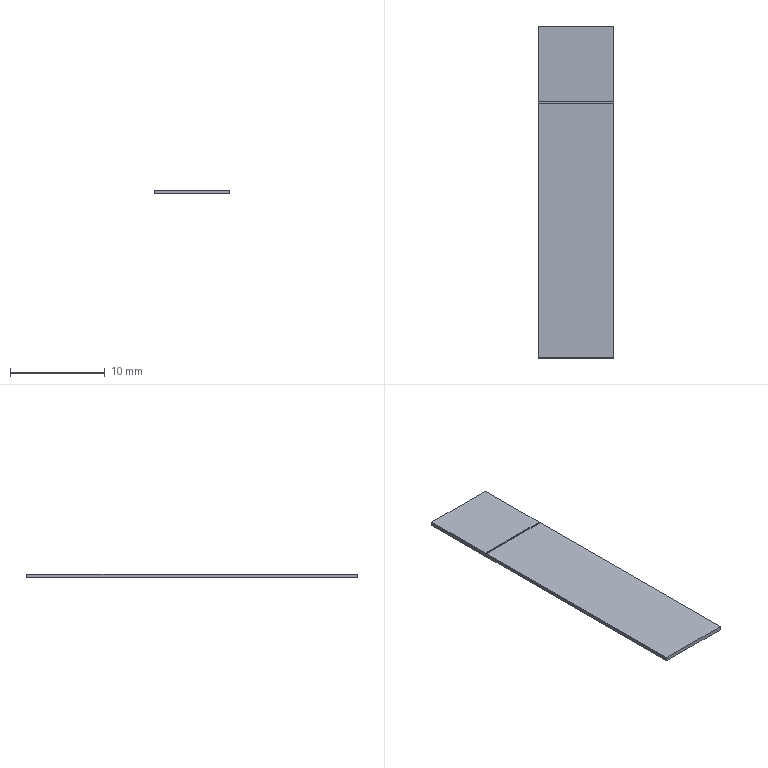Part | STEP file | 1 solid | 10 faces | box 8 x 35 x 0.41 mm | volume 114.776 mm3 | plane 10
STEP:
#1=CARTESIAN_POINT('',(0.,0.,0.));
#2=DIRECTION('',(0.,0.,1.));
#3=DIRECTION('',(1.,0.,0.));
#4=AXIS2_PLACEMENT_3D('',#1,#2,#3);
#5=CARTESIAN_POINT('',(4.,9.35,0.39));
#6=VERTEX_POINT('',#5);
#7=CARTESIAN_POINT('',(4.,9.5,0.39));
#8=VERTEX_POINT('',#7);
#9=CARTESIAN_POINT('',(4.,9.35,0.39));
#10=DIRECTION('',(0.,1.,0.));
#11=VECTOR('',#10,1.);
#12=LINE('',#9,#11);
#13=CARTESIAN_POINT('',(0.,0.,0.39));
#14=DIRECTION('',(0.,0.,-1.));
#15=DIRECTION('',(-1.,0.,0.));
#16=AXIS2_PLACEMENT_3D('',#13,#14,#15);
#17=PLANE('',#16);
#18=CARTESIAN_POINT('',(-4.,9.35));
#19=DIRECTION('',(0.,1.));
#20=VECTOR('',#19,1.);
#21=LINE('',#18,#20);
#22=(GEOMETRIC_REPRESENTATION_CONTEXT(2)PARAMETRIC_REPRESENTATION_CONTEXT()REPRESENTATION_CONTEXT('',''));
#23=DEFINITIONAL_REPRESENTATION('',(#21),#22);
#24=PCURVE('',#17,#23);
#25=CARTESIAN_POINT('',(4.,-17.5,0.41));
#26=DIRECTION('',(-1.,0.,0.));
#27=DIRECTION('',(0.,0.,1.));
#28=AXIS2_PLACEMENT_3D('',#25,#26,#27);
#29=PLANE('',#28);
#30=CARTESIAN_POINT('',(-0.02,26.85));
#31=DIRECTION('',(0.,1.));
#32=VECTOR('',#31,1.);
#33=LINE('',#30,#32);
#34=(GEOMETRIC_REPRESENTATION_CONTEXT(2)PARAMETRIC_REPRESENTATION_CONTEXT()REPRESENTATION_CONTEXT('',''));
#35=DEFINITIONAL_REPRESENTATION('',(#33),#34);
#36=PCURVE('',#29,#35);
#37=SURFACE_CURVE('',#12,(#24,#36),.PCURVE_S1.);
#38=EDGE_CURVE('',#6,#8,#37,.T.);
#39=ORIENTED_EDGE('',*,*,#38,.T.);
#40=CARTESIAN_POINT('',(-4.,9.5,0.39));
#41=VERTEX_POINT('',#40);
#42=CARTESIAN_POINT('',(-4.,9.5,0.39));
#43=DIRECTION('',(-1.,0.,0.));
#44=VECTOR('',#43,1.);
#45=LINE('',#42,#44);
#46=CARTESIAN_POINT('',(4.,9.5));
#47=DIRECTION('',(1.,0.));
#48=VECTOR('',#47,1.);
#49=LINE('',#46,#48);
#50=(GEOMETRIC_REPRESENTATION_CONTEXT(2)PARAMETRIC_REPRESENTATION_CONTEXT()REPRESENTATION_CONTEXT('',''));
#51=DEFINITIONAL_REPRESENTATION('',(#49),#50);
#52=PCURVE('',#17,#51);
#53=CARTESIAN_POINT('',(-4.,9.5,0.39));
#54=DIRECTION('',(0.,1.,0.));
#55=DIRECTION('',(0.,0.,1.));
#56=AXIS2_PLACEMENT_3D('',#53,#54,#55);
#57=PLANE('',#56);
#58=CARTESIAN_POINT('',(0.,0.));
#59=DIRECTION('',(0.,-1.));
#60=VECTOR('',#59,1.);
#61=LINE('',#58,#60);
#62=(GEOMETRIC_REPRESENTATION_CONTEXT(2)PARAMETRIC_REPRESENTATION_CONTEXT()REPRESENTATION_CONTEXT('',''));
#63=DEFINITIONAL_REPRESENTATION('',(#61),#62);
#64=PCURVE('',#57,#63);
#65=SURFACE_CURVE('',#45,(#52,#64),.PCURVE_S1.);
#66=EDGE_CURVE('',#8,#41,#65,.T.);
#67=ORIENTED_EDGE('',*,*,#66,.T.);
#68=CARTESIAN_POINT('',(-4.,9.35,0.39));
#69=VERTEX_POINT('',#68);
#70=CARTESIAN_POINT('',(-4.,9.35,0.39));
#71=DIRECTION('',(0.,-1.,0.));
#72=VECTOR('',#71,1.);
#73=LINE('',#70,#72);
#74=CARTESIAN_POINT('',(4.,9.35));
#75=DIRECTION('',(0.,-1.));
#76=VECTOR('',#75,1.);
#77=LINE('',#74,#76);
#78=(GEOMETRIC_REPRESENTATION_CONTEXT(2)PARAMETRIC_REPRESENTATION_CONTEXT()REPRESENTATION_CONTEXT('',''));
#79=DEFINITIONAL_REPRESENTATION('',(#77),#78);
#80=PCURVE('',#17,#79);
#81=CARTESIAN_POINT('',(-4.,-17.5,0.41));
#82=DIRECTION('',(1.,0.,0.));
#83=DIRECTION('',(0.,0.,-1.));
#84=AXIS2_PLACEMENT_3D('',#81,#82,#83);
#85=PLANE('',#84);
#86=CARTESIAN_POINT('',(0.02,26.85));
#87=DIRECTION('',(0.,-1.));
#88=VECTOR('',#87,1.);
#89=LINE('',#86,#88);
#90=(GEOMETRIC_REPRESENTATION_CONTEXT(2)PARAMETRIC_REPRESENTATION_CONTEXT()REPRESENTATION_CONTEXT('',''));
#91=DEFINITIONAL_REPRESENTATION('',(#89),#90);
#92=PCURVE('',#85,#91);
#93=SURFACE_CURVE('',#73,(#80,#92),.PCURVE_S1.);
#94=EDGE_CURVE('',#41,#69,#93,.T.);
#95=ORIENTED_EDGE('',*,*,#94,.T.);
#96=CARTESIAN_POINT('',(-4.,9.35,0.39));
#97=DIRECTION('',(1.,0.,0.));
#98=VECTOR('',#97,1.);
#99=LINE('',#96,#98);
#100=CARTESIAN_POINT('',(4.,9.35));
#101=DIRECTION('',(-1.,0.));
#102=VECTOR('',#101,1.);
#103=LINE('',#100,#102);
#104=(GEOMETRIC_REPRESENTATION_CONTEXT(2)PARAMETRIC_REPRESENTATION_CONTEXT()REPRESENTATION_CONTEXT('',''));
#105=DEFINITIONAL_REPRESENTATION('',(#103),#104);
#106=PCURVE('',#17,#105);
#107=CARTESIAN_POINT('',(-4.,9.35,0.39));
#108=DIRECTION('',(0.,-1.,0.));
#109=DIRECTION('',(0.,0.,-1.));
#110=AXIS2_PLACEMENT_3D('',#107,#108,#109);
#111=PLANE('',#110);
#112=CARTESIAN_POINT('',(0.,0.));
#113=DIRECTION('',(0.,1.));
#114=VECTOR('',#113,1.);
#115=LINE('',#112,#114);
#116=(GEOMETRIC_REPRESENTATION_CONTEXT(2)PARAMETRIC_REPRESENTATION_CONTEXT()REPRESENTATION_CONTEXT('',''));
#117=DEFINITIONAL_REPRESENTATION('',(#115),#116);
#118=PCURVE('',#111,#117);
#119=SURFACE_CURVE('',#99,(#106,#118),.PCURVE_S1.);
#120=EDGE_CURVE('',#69,#6,#119,.T.);
#121=ORIENTED_EDGE('',*,*,#120,.T.);
#122=EDGE_LOOP('',(#39,#67,#95,#121));
#123=FACE_BOUND('',#122,.T.);
#124=ADVANCED_FACE('',(#123),#17,.F.);
#125=CARTESIAN_POINT('',(4.,9.5,0.41));
#126=VERTEX_POINT('',#125);
#127=CARTESIAN_POINT('',(-4.,9.5,0.41));
#128=VERTEX_POINT('',#127);
#129=CARTESIAN_POINT('',(-4.,9.5,0.41));
#130=DIRECTION('',(-1.,0.,0.));
#131=VECTOR('',#130,1.);
#132=LINE('',#129,#131);
#133=CARTESIAN_POINT('',(0.02,0.));
#134=DIRECTION('',(0.,-1.));
#135=VECTOR('',#134,1.);
#136=LINE('',#133,#135);
#137=(GEOMETRIC_REPRESENTATION_CONTEXT(2)PARAMETRIC_REPRESENTATION_CONTEXT()REPRESENTATION_CONTEXT('',''));
#138=DEFINITIONAL_REPRESENTATION('',(#136),#137);
#139=PCURVE('',#57,#138);
#140=CARTESIAN_POINT('',(0.,0.,0.41));
#141=DIRECTION('',(0.,0.,-1.));
#142=DIRECTION('',(-1.,0.,0.));
#143=AXIS2_PLACEMENT_3D('',#140,#141,#142);
#144=PLANE('',#143);
#145=CARTESIAN_POINT('',(4.,9.5));
#146=DIRECTION('',(1.,0.));
#147=VECTOR('',#146,1.);
#148=LINE('',#145,#147);
#149=(GEOMETRIC_REPRESENTATION_CONTEXT(2)PARAMETRIC_REPRESENTATION_CONTEXT()REPRESENTATION_CONTEXT('',''));
#150=DEFINITIONAL_REPRESENTATION('',(#148),#149);
#151=PCURVE('',#144,#150);
#152=SURFACE_CURVE('',#132,(#139,#151),.PCURVE_S1.);
#153=EDGE_CURVE('',#126,#128,#152,.T.);
#154=ORIENTED_EDGE('',*,*,#153,.T.);
#155=CARTESIAN_POINT('',(-4.,9.5,0.39));
#156=DIRECTION('',(0.,0.,1.));
#157=VECTOR('',#156,1.);
#158=LINE('',#155,#157);
#159=CARTESIAN_POINT('',(0.,0.));
#160=DIRECTION('',(1.,0.));
#161=VECTOR('',#160,1.);
#162=LINE('',#159,#161);
#163=(GEOMETRIC_REPRESENTATION_CONTEXT(2)PARAMETRIC_REPRESENTATION_CONTEXT()REPRESENTATION_CONTEXT('',''));
#164=DEFINITIONAL_REPRESENTATION('',(#162),#163);
#165=PCURVE('',#57,#164);
#166=CARTESIAN_POINT('',(0.02,27.));
#167=DIRECTION('',(-1.,0.));
#168=VECTOR('',#167,1.);
#169=LINE('',#166,#168);
#170=(GEOMETRIC_REPRESENTATION_CONTEXT(2)PARAMETRIC_REPRESENTATION_CONTEXT()REPRESENTATION_CONTEXT('',''));
#171=DEFINITIONAL_REPRESENTATION('',(#169),#170);
#172=PCURVE('',#85,#171);
#173=SURFACE_CURVE('',#158,(#165,#172),.PCURVE_S1.);
#174=EDGE_CURVE('',#41,#128,#173,.T.);
#175=ORIENTED_EDGE('',*,*,#174,.F.);
#176=ORIENTED_EDGE('',*,*,#66,.F.);
#177=CARTESIAN_POINT('',(4.,9.5,0.39));
#178=DIRECTION('',(0.,0.,1.));
#179=VECTOR('',#178,1.);
#180=LINE('',#177,#179);
#181=CARTESIAN_POINT('',(0.,8.));
#182=DIRECTION('',(1.,0.));
#183=VECTOR('',#182,1.);
#184=LINE('',#181,#183);
#185=(GEOMETRIC_REPRESENTATION_CONTEXT(2)PARAMETRIC_REPRESENTATION_CONTEXT()REPRESENTATION_CONTEXT('',''));
#186=DEFINITIONAL_REPRESENTATION('',(#184),#185);
#187=PCURVE('',#57,#186);
#188=CARTESIAN_POINT('',(-0.02,27.));
#189=DIRECTION('',(1.,0.));
#190=VECTOR('',#189,1.);
#191=LINE('',#188,#190);
#192=(GEOMETRIC_REPRESENTATION_CONTEXT(2)PARAMETRIC_REPRESENTATION_CONTEXT()REPRESENTATION_CONTEXT('',''));
#193=DEFINITIONAL_REPRESENTATION('',(#191),#192);
#194=PCURVE('',#29,#193);
#195=SURFACE_CURVE('',#180,(#187,#194),.PCURVE_S1.);
#196=EDGE_CURVE('',#8,#126,#195,.T.);
#197=ORIENTED_EDGE('',*,*,#196,.T.);
#198=EDGE_LOOP('',(#154,#175,#176,#197));
#199=FACE_BOUND('',#198,.T.);
#200=ADVANCED_FACE('',(#199),#57,.F.);
#201=CARTESIAN_POINT('',(-4.,9.35,0.41));
#202=VERTEX_POINT('',#201);
#203=CARTESIAN_POINT('',(4.,9.35,0.41));
#204=VERTEX_POINT('',#203);
#205=CARTESIAN_POINT('',(-4.,9.35,0.41));
#206=DIRECTION('',(1.,0.,0.));
#207=VECTOR('',#206,1.);
#208=LINE('',#205,#207);
#209=CARTESIAN_POINT('',(-0.02,0.));
#210=DIRECTION('',(0.,1.));
#211=VECTOR('',#210,1.);
#212=LINE('',#209,#211);
#213=(GEOMETRIC_REPRESENTATION_CONTEXT(2)PARAMETRIC_REPRESENTATION_CONTEXT()REPRESENTATION_CONTEXT('',''));
#214=DEFINITIONAL_REPRESENTATION('',(#212),#213);
#215=PCURVE('',#111,#214);
#216=CARTESIAN_POINT('',(0.,0.,0.41));
#217=DIRECTION('',(0.,0.,-1.));
#218=DIRECTION('',(-1.,0.,0.));
#219=AXIS2_PLACEMENT_3D('',#216,#217,#218);
#220=PLANE('',#219);
#221=CARTESIAN_POINT('',(4.,9.35));
#222=DIRECTION('',(-1.,0.));
#223=VECTOR('',#222,1.);
#224=LINE('',#221,#223);
#225=(GEOMETRIC_REPRESENTATION_CONTEXT(2)PARAMETRIC_REPRESENTATION_CONTEXT()REPRESENTATION_CONTEXT('',''));
#226=DEFINITIONAL_REPRESENTATION('',(#224),#225);
#227=PCURVE('',#220,#226);
#228=SURFACE_CURVE('',#208,(#215,#227),.PCURVE_S1.);
#229=EDGE_CURVE('',#202,#204,#228,.T.);
#230=ORIENTED_EDGE('',*,*,#229,.T.);
#231=CARTESIAN_POINT('',(4.,9.35,0.39));
#232=DIRECTION('',(0.,0.,1.));
#233=VECTOR('',#232,1.);
#234=LINE('',#231,#233);
#235=CARTESIAN_POINT('',(0.,8.));
#236=DIRECTION('',(-1.,0.));
#237=VECTOR('',#236,1.);
#238=LINE('',#235,#237);
#239=(GEOMETRIC_REPRESENTATION_CONTEXT(2)PARAMETRIC_REPRESENTATION_CONTEXT()REPRESENTATION_CONTEXT('',''));
#240=DEFINITIONAL_REPRESENTATION('',(#238),#239);
#241=PCURVE('',#111,#240);
#242=CARTESIAN_POINT('',(-0.02,26.85));
#243=DIRECTION('',(1.,0.));
#244=VECTOR('',#243,1.);
#245=LINE('',#242,#244);
#246=(GEOMETRIC_REPRESENTATION_CONTEXT(2)PARAMETRIC_REPRESENTATION_CONTEXT()REPRESENTATION_CONTEXT('',''));
#247=DEFINITIONAL_REPRESENTATION('',(#245),#246);
#248=PCURVE('',#29,#247);
#249=SURFACE_CURVE('',#234,(#241,#248),.PCURVE_S1.);
#250=EDGE_CURVE('',#6,#204,#249,.T.);
#251=ORIENTED_EDGE('',*,*,#250,.F.);
#252=ORIENTED_EDGE('',*,*,#120,.F.);
#253=CARTESIAN_POINT('',(-4.,9.35,0.39));
#254=DIRECTION('',(0.,0.,1.));
#255=VECTOR('',#254,1.);
#256=LINE('',#253,#255);
#257=CARTESIAN_POINT('',(0.,0.));
#258=DIRECTION('',(-1.,0.));
#259=VECTOR('',#258,1.);
#260=LINE('',#257,#259);
#261=(GEOMETRIC_REPRESENTATION_CONTEXT(2)PARAMETRIC_REPRESENTATION_CONTEXT()REPRESENTATION_CONTEXT('',''));
#262=DEFINITIONAL_REPRESENTATION('',(#260),#261);
#263=PCURVE('',#111,#262);
#264=CARTESIAN_POINT('',(0.02,26.85));
#265=DIRECTION('',(-1.,0.));
#266=VECTOR('',#265,1.);
#267=LINE('',#264,#266);
#268=(GEOMETRIC_REPRESENTATION_CONTEXT(2)PARAMETRIC_REPRESENTATION_CONTEXT()REPRESENTATION_CONTEXT('',''));
#269=DEFINITIONAL_REPRESENTATION('',(#267),#268);
#270=PCURVE('',#85,#269);
#271=SURFACE_CURVE('',#256,(#263,#270),.PCURVE_S1.);
#272=EDGE_CURVE('',#69,#202,#271,.T.);
#273=ORIENTED_EDGE('',*,*,#272,.T.);
#274=EDGE_LOOP('',(#230,#251,#252,#273));
#275=FACE_BOUND('',#274,.T.);
#276=ADVANCED_FACE('',(#275),#111,.F.);
#277=CARTESIAN_POINT('',(4.,-17.5,0.));
#278=VERTEX_POINT('',#277);
#279=CARTESIAN_POINT('',(4.,17.5,0.));
#280=VERTEX_POINT('',#279);
#281=CARTESIAN_POINT('',(4.,-17.5,0.));
#282=DIRECTION('',(0.,1.,0.));
#283=VECTOR('',#282,1.);
#284=LINE('',#281,#283);
#285=CARTESIAN_POINT('',(0.,0.,0.));
#286=DIRECTION('',(0.,0.,-1.));
#287=DIRECTION('',(-1.,0.,0.));
#288=AXIS2_PLACEMENT_3D('',#285,#286,#287);
#289=PLANE('',#288);
#290=CARTESIAN_POINT('',(-4.,-17.5));
#291=DIRECTION('',(0.,1.));
#292=VECTOR('',#291,1.);
#293=LINE('',#290,#292);
#294=(GEOMETRIC_REPRESENTATION_CONTEXT(2)PARAMETRIC_REPRESENTATION_CONTEXT()REPRESENTATION_CONTEXT('',''));
#295=DEFINITIONAL_REPRESENTATION('',(#293),#294);
#296=PCURVE('',#289,#295);
#297=CARTESIAN_POINT('',(-0.41,0.));
#298=DIRECTION('',(0.,1.));
#299=VECTOR('',#298,1.);
#300=LINE('',#297,#299);
#301=(GEOMETRIC_REPRESENTATION_CONTEXT(2)PARAMETRIC_REPRESENTATION_CONTEXT()REPRESENTATION_CONTEXT('',''));
#302=DEFINITIONAL_REPRESENTATION('',(#300),#301);
#303=PCURVE('',#29,#302);
#304=SURFACE_CURVE('',#284,(#296,#303),.PCURVE_S1.);
#305=EDGE_CURVE('',#278,#280,#304,.T.);
#306=ORIENTED_EDGE('',*,*,#305,.F.);
#307=CARTESIAN_POINT('',(-4.,-17.5,0.));
#308=VERTEX_POINT('',#307);
#309=CARTESIAN_POINT('',(-4.,-17.5,0.));
#310=DIRECTION('',(1.,0.,0.));
#311=VECTOR('',#310,1.);
#312=LINE('',#309,#311);
#313=CARTESIAN_POINT('',(4.,-17.5));
#314=DIRECTION('',(-1.,0.));
#315=VECTOR('',#314,1.);
#316=LINE('',#313,#315);
#317=(GEOMETRIC_REPRESENTATION_CONTEXT(2)PARAMETRIC_REPRESENTATION_CONTEXT()REPRESENTATION_CONTEXT('',''));
#318=DEFINITIONAL_REPRESENTATION('',(#316),#317);
#319=PCURVE('',#289,#318);
#320=CARTESIAN_POINT('',(-4.,-17.5,0.41));
#321=DIRECTION('',(0.,1.,0.));
#322=DIRECTION('',(0.,0.,1.));
#323=AXIS2_PLACEMENT_3D('',#320,#321,#322);
#324=PLANE('',#323);
#325=CARTESIAN_POINT('',(-0.41,0.));
#326=DIRECTION('',(0.,1.));
#327=VECTOR('',#326,1.);
#328=LINE('',#325,#327);
#329=(GEOMETRIC_REPRESENTATION_CONTEXT(2)PARAMETRIC_REPRESENTATION_CONTEXT()REPRESENTATION_CONTEXT('',''));
#330=DEFINITIONAL_REPRESENTATION('',(#328),#329);
#331=PCURVE('',#324,#330);
#332=SURFACE_CURVE('',#312,(#319,#331),.PCURVE_S1.);
#333=EDGE_CURVE('',#308,#278,#332,.T.);
#334=ORIENTED_EDGE('',*,*,#333,.F.);
#335=CARTESIAN_POINT('',(-4.,17.5,0.));
#336=VERTEX_POINT('',#335);
#337=CARTESIAN_POINT('',(-4.,-17.5,0.));
#338=DIRECTION('',(0.,-1.,0.));
#339=VECTOR('',#338,1.);
#340=LINE('',#337,#339);
#341=CARTESIAN_POINT('',(4.,-17.5));
#342=DIRECTION('',(0.,-1.));
#343=VECTOR('',#342,1.);
#344=LINE('',#341,#343);
#345=(GEOMETRIC_REPRESENTATION_CONTEXT(2)PARAMETRIC_REPRESENTATION_CONTEXT()REPRESENTATION_CONTEXT('',''));
#346=DEFINITIONAL_REPRESENTATION('',(#344),#345);
#347=PCURVE('',#289,#346);
#348=CARTESIAN_POINT('',(0.41,0.));
#349=DIRECTION('',(0.,-1.));
#350=VECTOR('',#349,1.);
#351=LINE('',#348,#350);
#352=(GEOMETRIC_REPRESENTATION_CONTEXT(2)PARAMETRIC_REPRESENTATION_CONTEXT()REPRESENTATION_CONTEXT('',''));
#353=DEFINITIONAL_REPRESENTATION('',(#351),#352);
#354=PCURVE('',#85,#353);
#355=SURFACE_CURVE('',#340,(#347,#354),.PCURVE_S1.);
#356=EDGE_CURVE('',#336,#308,#355,.T.);
#357=ORIENTED_EDGE('',*,*,#356,.F.);
#358=CARTESIAN_POINT('',(-4.,17.5,0.));
#359=DIRECTION('',(-1.,0.,0.));
#360=VECTOR('',#359,1.);
#361=LINE('',#358,#360);
#362=CARTESIAN_POINT('',(4.,17.5));
#363=DIRECTION('',(1.,0.));
#364=VECTOR('',#363,1.);
#365=LINE('',#362,#364);
#366=(GEOMETRIC_REPRESENTATION_CONTEXT(2)PARAMETRIC_REPRESENTATION_CONTEXT()REPRESENTATION_CONTEXT('',''));
#367=DEFINITIONAL_REPRESENTATION('',(#365),#366);
#368=PCURVE('',#289,#367);
#369=CARTESIAN_POINT('',(-4.,17.5,0.41));
#370=DIRECTION('',(0.,-1.,0.));
#371=DIRECTION('',(0.,0.,-1.));
#372=AXIS2_PLACEMENT_3D('',#369,#370,#371);
#373=PLANE('',#372);
#374=CARTESIAN_POINT('',(0.41,0.));
#375=DIRECTION('',(0.,-1.));
#376=VECTOR('',#375,1.);
#377=LINE('',#374,#376);
#378=(GEOMETRIC_REPRESENTATION_CONTEXT(2)PARAMETRIC_REPRESENTATION_CONTEXT()REPRESENTATION_CONTEXT('',''));
#379=DEFINITIONAL_REPRESENTATION('',(#377),#378);
#380=PCURVE('',#373,#379);
#381=SURFACE_CURVE('',#361,(#368,#380),.PCURVE_S1.);
#382=EDGE_CURVE('',#280,#336,#381,.T.);
#383=ORIENTED_EDGE('',*,*,#382,.F.);
#384=EDGE_LOOP('',(#306,#334,#357,#383));
#385=FACE_BOUND('',#384,.T.);
#386=ADVANCED_FACE('',(#385),#289,.T.);
#387=CARTESIAN_POINT('',(-4.,17.5,0.41));
#388=VERTEX_POINT('',#387);
#389=CARTESIAN_POINT('',(-4.,-17.5,0.41));
#390=DIRECTION('',(0.,-1.,0.));
#391=VECTOR('',#390,1.);
#392=LINE('',#389,#391);
#393=CARTESIAN_POINT('',(4.,-17.5));
#394=DIRECTION('',(0.,-1.));
#395=VECTOR('',#394,1.);
#396=LINE('',#393,#395);
#397=(GEOMETRIC_REPRESENTATION_CONTEXT(2)PARAMETRIC_REPRESENTATION_CONTEXT()REPRESENTATION_CONTEXT('',''));
#398=DEFINITIONAL_REPRESENTATION('',(#396),#397);
#399=PCURVE('',#144,#398);
#400=CARTESIAN_POINT('',(0.,0.));
#401=DIRECTION('',(0.,-1.));
#402=VECTOR('',#401,1.);
#403=LINE('',#400,#402);
#404=(GEOMETRIC_REPRESENTATION_CONTEXT(2)PARAMETRIC_REPRESENTATION_CONTEXT()REPRESENTATION_CONTEXT('',''));
#405=DEFINITIONAL_REPRESENTATION('',(#403),#404);
#406=PCURVE('',#85,#405);
#407=SURFACE_CURVE('',#392,(#399,#406),.PCURVE_S1.);
#408=EDGE_CURVE('',#388,#128,#407,.T.);
#409=ORIENTED_EDGE('',*,*,#408,.T.);
#410=ORIENTED_EDGE('',*,*,#153,.F.);
#411=CARTESIAN_POINT('',(4.,17.5,0.41));
#412=VERTEX_POINT('',#411);
#413=CARTESIAN_POINT('',(4.,-17.5,0.41));
#414=DIRECTION('',(0.,1.,0.));
#415=VECTOR('',#414,1.);
#416=LINE('',#413,#415);
#417=CARTESIAN_POINT('',(-4.,-17.5));
#418=DIRECTION('',(0.,1.));
#419=VECTOR('',#418,1.);
#420=LINE('',#417,#419);
#421=(GEOMETRIC_REPRESENTATION_CONTEXT(2)PARAMETRIC_REPRESENTATION_CONTEXT()REPRESENTATION_CONTEXT('',''));
#422=DEFINITIONAL_REPRESENTATION('',(#420),#421);
#423=PCURVE('',#144,#422);
#424=CARTESIAN_POINT('',(0.,0.));
#425=DIRECTION('',(0.,1.));
#426=VECTOR('',#425,1.);
#427=LINE('',#424,#426);
#428=(GEOMETRIC_REPRESENTATION_CONTEXT(2)PARAMETRIC_REPRESENTATION_CONTEXT()REPRESENTATION_CONTEXT('',''));
#429=DEFINITIONAL_REPRESENTATION('',(#427),#428);
#430=PCURVE('',#29,#429);
#431=SURFACE_CURVE('',#416,(#423,#430),.PCURVE_S1.);
#432=EDGE_CURVE('',#126,#412,#431,.T.);
#433=ORIENTED_EDGE('',*,*,#432,.T.);
#434=CARTESIAN_POINT('',(-4.,17.5,0.41));
#435=DIRECTION('',(-1.,0.,0.));
#436=VECTOR('',#435,1.);
#437=LINE('',#434,#436);
#438=CARTESIAN_POINT('',(4.,17.5));
#439=DIRECTION('',(1.,0.));
#440=VECTOR('',#439,1.);
#441=LINE('',#438,#440);
#442=(GEOMETRIC_REPRESENTATION_CONTEXT(2)PARAMETRIC_REPRESENTATION_CONTEXT()REPRESENTATION_CONTEXT('',''));
#443=DEFINITIONAL_REPRESENTATION('',(#441),#442);
#444=PCURVE('',#144,#443);
#445=CARTESIAN_POINT('',(0.,0.));
#446=DIRECTION('',(0.,-1.));
#447=VECTOR('',#446,1.);
#448=LINE('',#445,#447);
#449=(GEOMETRIC_REPRESENTATION_CONTEXT(2)PARAMETRIC_REPRESENTATION_CONTEXT()REPRESENTATION_CONTEXT('',''));
#450=DEFINITIONAL_REPRESENTATION('',(#448),#449);
#451=PCURVE('',#373,#450);
#452=SURFACE_CURVE('',#437,(#444,#451),.PCURVE_S1.);
#453=EDGE_CURVE('',#412,#388,#452,.T.);
#454=ORIENTED_EDGE('',*,*,#453,.T.);
#455=EDGE_LOOP('',(#409,#410,#433,#454));
#456=FACE_BOUND('',#455,.T.);
#457=ADVANCED_FACE('',(#456),#144,.F.);
#458=ORIENTED_EDGE('',*,*,#333,.T.);
#459=CARTESIAN_POINT('',(4.,-17.5,0.41));
#460=VERTEX_POINT('',#459);
#461=CARTESIAN_POINT('',(4.,-17.5,0.41));
#462=DIRECTION('',(0.,0.,-1.));
#463=VECTOR('',#462,1.);
#464=LINE('',#461,#463);
#465=CARTESIAN_POINT('',(0.,8.));
#466=DIRECTION('',(-1.,0.));
#467=VECTOR('',#466,1.);
#468=LINE('',#465,#467);
#469=(GEOMETRIC_REPRESENTATION_CONTEXT(2)PARAMETRIC_REPRESENTATION_CONTEXT()REPRESENTATION_CONTEXT('',''));
#470=DEFINITIONAL_REPRESENTATION('',(#468),#469);
#471=PCURVE('',#324,#470);
#472=CARTESIAN_POINT('',(0.,0.));
#473=DIRECTION('',(-1.,0.));
#474=VECTOR('',#473,1.);
#475=LINE('',#472,#474);
#476=(GEOMETRIC_REPRESENTATION_CONTEXT(2)PARAMETRIC_REPRESENTATION_CONTEXT()REPRESENTATION_CONTEXT('',''));
#477=DEFINITIONAL_REPRESENTATION('',(#475),#476);
#478=PCURVE('',#29,#477);
#479=SURFACE_CURVE('',#464,(#471,#478),.PCURVE_S1.);
#480=EDGE_CURVE('',#460,#278,#479,.T.);
#481=ORIENTED_EDGE('',*,*,#480,.F.);
#482=CARTESIAN_POINT('',(-4.,-17.5,0.41));
#483=VERTEX_POINT('',#482);
#484=CARTESIAN_POINT('',(-4.,-17.5,0.41));
#485=DIRECTION('',(1.,0.,0.));
#486=VECTOR('',#485,1.);
#487=LINE('',#484,#486);
#488=CARTESIAN_POINT('',(0.,0.));
#489=DIRECTION('',(0.,1.));
#490=VECTOR('',#489,1.);
#491=LINE('',#488,#490);
#492=(GEOMETRIC_REPRESENTATION_CONTEXT(2)PARAMETRIC_REPRESENTATION_CONTEXT()REPRESENTATION_CONTEXT('',''));
#493=DEFINITIONAL_REPRESENTATION('',(#491),#492);
#494=PCURVE('',#324,#493);
#495=CARTESIAN_POINT('',(4.,-17.5));
#496=DIRECTION('',(-1.,0.));
#497=VECTOR('',#496,1.);
#498=LINE('',#495,#497);
#499=(GEOMETRIC_REPRESENTATION_CONTEXT(2)PARAMETRIC_REPRESENTATION_CONTEXT()REPRESENTATION_CONTEXT('',''));
#500=DEFINITIONAL_REPRESENTATION('',(#498),#499);
#501=PCURVE('',#220,#500);
#502=SURFACE_CURVE('',#487,(#494,#501),.PCURVE_S1.);
#503=EDGE_CURVE('',#483,#460,#502,.T.);
#504=ORIENTED_EDGE('',*,*,#503,.F.);
#505=CARTESIAN_POINT('',(-4.,-17.5,0.41));
#506=DIRECTION('',(0.,0.,-1.));
#507=VECTOR('',#506,1.);
#508=LINE('',#505,#507);
#509=CARTESIAN_POINT('',(0.,0.));
#510=DIRECTION('',(-1.,0.));
#511=VECTOR('',#510,1.);
#512=LINE('',#509,#511);
#513=(GEOMETRIC_REPRESENTATION_CONTEXT(2)PARAMETRIC_REPRESENTATION_CONTEXT()REPRESENTATION_CONTEXT('',''));
#514=DEFINITIONAL_REPRESENTATION('',(#512),#513);
#515=PCURVE('',#324,#514);
#516=CARTESIAN_POINT('',(0.,0.));
#517=DIRECTION('',(1.,0.));
#518=VECTOR('',#517,1.);
#519=LINE('',#516,#518);
#520=(GEOMETRIC_REPRESENTATION_CONTEXT(2)PARAMETRIC_REPRESENTATION_CONTEXT()REPRESENTATION_CONTEXT('',''));
#521=DEFINITIONAL_REPRESENTATION('',(#519),#520);
#522=PCURVE('',#85,#521);
#523=SURFACE_CURVE('',#508,(#515,#522),.PCURVE_S1.);
#524=EDGE_CURVE('',#483,#308,#523,.T.);
#525=ORIENTED_EDGE('',*,*,#524,.T.);
#526=EDGE_LOOP('',(#458,#481,#504,#525));
#527=FACE_BOUND('',#526,.T.);
#528=ADVANCED_FACE('',(#527),#324,.F.);
#529=CARTESIAN_POINT('',(-4.,-17.5,0.41));
#530=DIRECTION('',(0.,-1.,0.));
#531=VECTOR('',#530,1.);
#532=LINE('',#529,#531);
#533=CARTESIAN_POINT('',(0.,0.));
#534=DIRECTION('',(0.,-1.));
#535=VECTOR('',#534,1.);
#536=LINE('',#533,#535);
#537=(GEOMETRIC_REPRESENTATION_CONTEXT(2)PARAMETRIC_REPRESENTATION_CONTEXT()REPRESENTATION_CONTEXT('',''));
#538=DEFINITIONAL_REPRESENTATION('',(#536),#537);
#539=PCURVE('',#85,#538);
#540=CARTESIAN_POINT('',(4.,-17.5));
#541=DIRECTION('',(0.,-1.));
#542=VECTOR('',#541,1.);
#543=LINE('',#540,#542);
#544=(GEOMETRIC_REPRESENTATION_CONTEXT(2)PARAMETRIC_REPRESENTATION_CONTEXT()REPRESENTATION_CONTEXT('',''));
#545=DEFINITIONAL_REPRESENTATION('',(#543),#544);
#546=PCURVE('',#220,#545);
#547=SURFACE_CURVE('',#532,(#539,#546),.PCURVE_S1.);
#548=EDGE_CURVE('',#202,#483,#547,.T.);
#549=ORIENTED_EDGE('',*,*,#548,.F.);
#550=ORIENTED_EDGE('',*,*,#272,.F.);
#551=ORIENTED_EDGE('',*,*,#94,.F.);
#552=ORIENTED_EDGE('',*,*,#174,.T.);
#553=ORIENTED_EDGE('',*,*,#408,.F.);
#554=CARTESIAN_POINT('',(-4.,17.5,0.41));
#555=DIRECTION('',(0.,0.,-1.));
#556=VECTOR('',#555,1.);
#557=LINE('',#554,#556);
#558=CARTESIAN_POINT('',(0.,35.));
#559=DIRECTION('',(1.,0.));
#560=VECTOR('',#559,1.);
#561=LINE('',#558,#560);
#562=(GEOMETRIC_REPRESENTATION_CONTEXT(2)PARAMETRIC_REPRESENTATION_CONTEXT()REPRESENTATION_CONTEXT('',''));
#563=DEFINITIONAL_REPRESENTATION('',(#561),#562);
#564=PCURVE('',#85,#563);
#565=CARTESIAN_POINT('',(0.,0.));
#566=DIRECTION('',(1.,0.));
#567=VECTOR('',#566,1.);
#568=LINE('',#565,#567);
#569=(GEOMETRIC_REPRESENTATION_CONTEXT(2)PARAMETRIC_REPRESENTATION_CONTEXT()REPRESENTATION_CONTEXT('',''));
#570=DEFINITIONAL_REPRESENTATION('',(#568),#569);
#571=PCURVE('',#373,#570);
#572=SURFACE_CURVE('',#557,(#564,#571),.PCURVE_S1.);
#573=EDGE_CURVE('',#388,#336,#572,.T.);
#574=ORIENTED_EDGE('',*,*,#573,.T.);
#575=ORIENTED_EDGE('',*,*,#356,.T.);
#576=ORIENTED_EDGE('',*,*,#524,.F.);
#577=EDGE_LOOP('',(#549,#550,#551,#552,#553,#574,#575,#576));
#578=FACE_BOUND('',#577,.T.);
#579=ADVANCED_FACE('',(#578),#85,.F.);
#580=ORIENTED_EDGE('',*,*,#382,.T.);
#581=ORIENTED_EDGE('',*,*,#573,.F.);
#582=ORIENTED_EDGE('',*,*,#453,.F.);
#583=CARTESIAN_POINT('',(4.,17.5,0.41));
#584=DIRECTION('',(0.,0.,-1.));
#585=VECTOR('',#584,1.);
#586=LINE('',#583,#585);
#587=CARTESIAN_POINT('',(0.,8.));
#588=DIRECTION('',(1.,0.));
#589=VECTOR('',#588,1.);
#590=LINE('',#587,#589);
#591=(GEOMETRIC_REPRESENTATION_CONTEXT(2)PARAMETRIC_REPRESENTATION_CONTEXT()REPRESENTATION_CONTEXT('',''));
#592=DEFINITIONAL_REPRESENTATION('',(#590),#591);
#593=PCURVE('',#373,#592);
#594=CARTESIAN_POINT('',(0.,35.));
#595=DIRECTION('',(-1.,0.));
#596=VECTOR('',#595,1.);
#597=LINE('',#594,#596);
#598=(GEOMETRIC_REPRESENTATION_CONTEXT(2)PARAMETRIC_REPRESENTATION_CONTEXT()REPRESENTATION_CONTEXT('',''));
#599=DEFINITIONAL_REPRESENTATION('',(#597),#598);
#600=PCURVE('',#29,#599);
#601=SURFACE_CURVE('',#586,(#593,#600),.PCURVE_S1.);
#602=EDGE_CURVE('',#412,#280,#601,.T.);
#603=ORIENTED_EDGE('',*,*,#602,.T.);
#604=EDGE_LOOP('',(#580,#581,#582,#603));
#605=FACE_BOUND('',#604,.T.);
#606=ADVANCED_FACE('',(#605),#373,.F.);
#607=ORIENTED_EDGE('',*,*,#38,.F.);
#608=ORIENTED_EDGE('',*,*,#250,.T.);
#609=CARTESIAN_POINT('',(4.,-17.5,0.41));
#610=DIRECTION('',(0.,1.,0.));
#611=VECTOR('',#610,1.);
#612=LINE('',#609,#611);
#613=CARTESIAN_POINT('',(0.,0.));
#614=DIRECTION('',(0.,1.));
#615=VECTOR('',#614,1.);
#616=LINE('',#613,#615);
#617=(GEOMETRIC_REPRESENTATION_CONTEXT(2)PARAMETRIC_REPRESENTATION_CONTEXT()REPRESENTATION_CONTEXT('',''));
#618=DEFINITIONAL_REPRESENTATION('',(#616),#617);
#619=PCURVE('',#29,#618);
#620=CARTESIAN_POINT('',(-4.,-17.5));
#621=DIRECTION('',(0.,1.));
#622=VECTOR('',#621,1.);
#623=LINE('',#620,#622);
#624=(GEOMETRIC_REPRESENTATION_CONTEXT(2)PARAMETRIC_REPRESENTATION_CONTEXT()REPRESENTATION_CONTEXT('',''));
#625=DEFINITIONAL_REPRESENTATION('',(#623),#624);
#626=PCURVE('',#220,#625);
#627=SURFACE_CURVE('',#612,(#619,#626),.PCURVE_S1.);
#628=EDGE_CURVE('',#460,#204,#627,.T.);
#629=ORIENTED_EDGE('',*,*,#628,.F.);
#630=ORIENTED_EDGE('',*,*,#480,.T.);
#631=ORIENTED_EDGE('',*,*,#305,.T.);
#632=ORIENTED_EDGE('',*,*,#602,.F.);
#633=ORIENTED_EDGE('',*,*,#432,.F.);
#634=ORIENTED_EDGE('',*,*,#196,.F.);
#635=EDGE_LOOP('',(#607,#608,#629,#630,#631,#632,#633,#634));
#636=FACE_BOUND('',#635,.T.);
#637=ADVANCED_FACE('',(#636),#29,.F.);
#638=ORIENTED_EDGE('',*,*,#628,.T.);
#639=ORIENTED_EDGE('',*,*,#229,.F.);
#640=ORIENTED_EDGE('',*,*,#548,.T.);
#641=ORIENTED_EDGE('',*,*,#503,.T.);
#642=EDGE_LOOP('',(#638,#639,#640,#641));
#643=FACE_BOUND('',#642,.T.);
#644=ADVANCED_FACE('',(#643),#220,.F.);
#645=CLOSED_SHELL('',(#124,#200,#276,#386,#457,#528,#579,#606,#637,#644));
#646=MANIFOLD_SOLID_BREP('',#645);
#647=(LENGTH_UNIT()NAMED_UNIT(*)SI_UNIT(.MILLI.,.METRE.));
#648=UNCERTAINTY_MEASURE_WITH_UNIT(LENGTH_MEASURE(0.0000001),#647,'','');
#649=(NAMED_UNIT(*)PLANE_ANGLE_UNIT()SI_UNIT($,.RADIAN.));
#650=(NAMED_UNIT(*)SI_UNIT($,.STERADIAN.)SOLID_ANGLE_UNIT());
#651=(GEOMETRIC_REPRESENTATION_CONTEXT(3)GLOBAL_UNCERTAINTY_ASSIGNED_CONTEXT((#648))GLOBAL_UNIT_ASSIGNED_CONTEXT((#647,#649,#650))REPRESENTATION_CONTEXT('',''));
#652=ADVANCED_BREP_SHAPE_REPRESENTATION('',(#4,#646),#651);